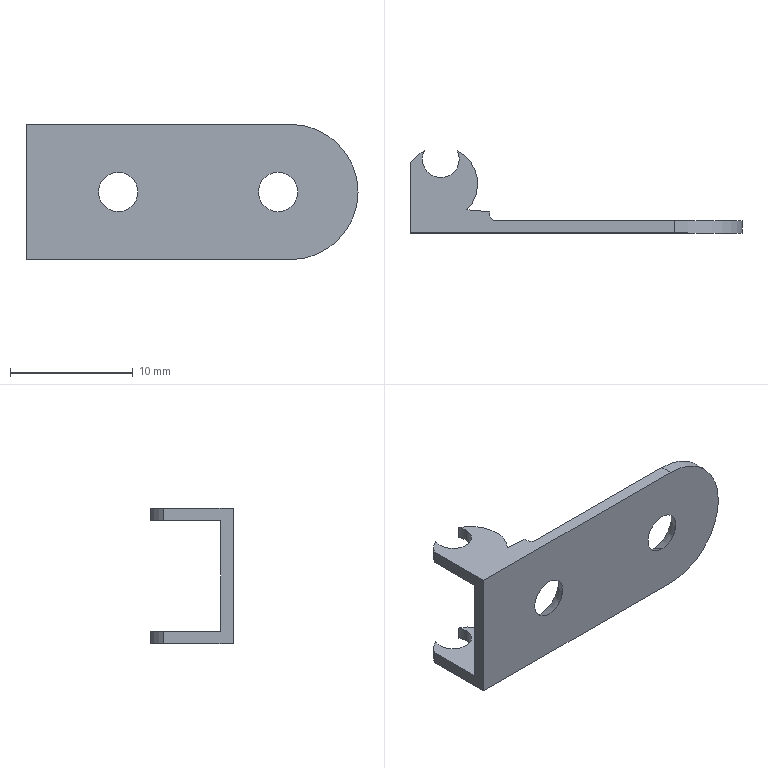Part | SolidWorks | features RefAxis 3, ICE 2, RevCut 2, 3DProfileFeature 1, Extrusion 1 | 1 solid | 28 faces | box 27 x 6.688 x 11 mm | volume 310.781 mm3 | cylinder 13 | plane 11 | cone 4 | commonest cylinder face diameters 3 x6 6 x4 1 x2 11 x1
STEP:
#1=CARTESIAN_POINT('',(20.5,0.,-1.6));
#2=VERTEX_POINT('',#1);
#3=CARTESIAN_POINT('',(20.5,0.,1.6));
#4=VERTEX_POINT('',#3);
#5=CARTESIAN_POINT('',(20.5,0.,0.));
#6=DIRECTION('',(0.,1.,0.));
#7=DIRECTION('',(0.,0.,1.));
#8=AXIS2_PLACEMENT_3D('',#5,#6,#7);
#9=CIRCLE('',#8,1.6);
#10=EDGE_CURVE('',#2,#4,#9,.T.);
#11=ORIENTED_EDGE('',*,*,#10,.F.);
#12=CARTESIAN_POINT('',(20.5,1.,-2.1));
#13=VERTEX_POINT('',#12);
#14=CARTESIAN_POINT('',(20.5,0.,-1.6));
#15=DIRECTION('',(0.,0.8944,-0.4472));
#16=VECTOR('',#15,1000.);
#17=LINE('',#14,#16);
#18=EDGE_CURVE('',#2,#13,#17,.T.);
#19=ORIENTED_EDGE('',*,*,#18,.T.);
#20=CARTESIAN_POINT('',(20.5,1.,2.1));
#21=VERTEX_POINT('',#20);
#22=CARTESIAN_POINT('',(20.5,1.,0.));
#23=DIRECTION('',(0.,1.,0.));
#24=DIRECTION('',(0.,0.,1.));
#25=AXIS2_PLACEMENT_3D('',#22,#23,#24);
#26=CIRCLE('',#25,2.1);
#27=EDGE_CURVE('',#13,#21,#26,.T.);
#28=ORIENTED_EDGE('',*,*,#27,.T.);
#29=CARTESIAN_POINT('',(20.5,0.,1.6));
#30=DIRECTION('',(0.,0.8944,0.4472));
#31=VECTOR('',#30,1000.);
#32=LINE('',#29,#31);
#33=EDGE_CURVE('',#4,#21,#32,.T.);
#34=ORIENTED_EDGE('',*,*,#33,.F.);
#35=EDGE_LOOP('',(#11,#19,#28,#34));
#36=FACE_OUTER_BOUND('',#35,.T.);
#37=CARTESIAN_POINT('',(20.5,0.,0.));
#38=DIRECTION('',(0.,1.,0.));
#39=DIRECTION('',(0.,0.,1.));
#40=AXIS2_PLACEMENT_3D('',#37,#38,#39);
#41=CONICAL_SURFACE('',#40,1.6,0.4636);
#42=ADVANCED_FACE('',(#36),#41,.F.);
#43=CARTESIAN_POINT('',(7.5,0.,-1.6));
#44=VERTEX_POINT('',#43);
#45=CARTESIAN_POINT('',(7.5,0.,1.6));
#46=VERTEX_POINT('',#45);
#47=CARTESIAN_POINT('',(7.5,0.,0.));
#48=DIRECTION('',(0.,1.,0.));
#49=DIRECTION('',(0.,0.,1.));
#50=AXIS2_PLACEMENT_3D('',#47,#48,#49);
#51=CIRCLE('',#50,1.6);
#52=EDGE_CURVE('',#44,#46,#51,.T.);
#53=ORIENTED_EDGE('',*,*,#52,.F.);
#54=CARTESIAN_POINT('',(7.5,1.,-2.1));
#55=VERTEX_POINT('',#54);
#56=CARTESIAN_POINT('',(7.5,0.,-1.6));
#57=DIRECTION('',(0.,0.8944,-0.4472));
#58=VECTOR('',#57,1000.);
#59=LINE('',#56,#58);
#60=EDGE_CURVE('',#44,#55,#59,.T.);
#61=ORIENTED_EDGE('',*,*,#60,.T.);
#62=CARTESIAN_POINT('',(7.5,1.,2.1));
#63=VERTEX_POINT('',#62);
#64=CARTESIAN_POINT('',(7.5,1.,0.));
#65=DIRECTION('',(0.,1.,0.));
#66=DIRECTION('',(0.,0.,1.));
#67=AXIS2_PLACEMENT_3D('',#64,#65,#66);
#68=CIRCLE('',#67,2.1);
#69=EDGE_CURVE('',#55,#63,#68,.T.);
#70=ORIENTED_EDGE('',*,*,#69,.T.);
#71=CARTESIAN_POINT('',(7.5,0.,1.6));
#72=DIRECTION('',(0.,0.8944,0.4472));
#73=VECTOR('',#72,1000.);
#74=LINE('',#71,#73);
#75=EDGE_CURVE('',#46,#63,#74,.T.);
#76=ORIENTED_EDGE('',*,*,#75,.F.);
#77=EDGE_LOOP('',(#53,#61,#70,#76));
#78=FACE_OUTER_BOUND('',#77,.T.);
#79=CARTESIAN_POINT('',(7.5,0.,0.));
#80=DIRECTION('',(0.,1.,0.));
#81=DIRECTION('',(0.,0.,1.));
#82=AXIS2_PLACEMENT_3D('',#79,#80,#81);
#83=CONICAL_SURFACE('',#82,1.6,0.4636);
#84=ADVANCED_FACE('',(#78),#83,.F.);
#85=CARTESIAN_POINT('',(4.,6.,-4.5));
#86=VERTEX_POINT('',#85);
#87=CARTESIAN_POINT('',(1.,6.,-4.5));
#88=VERTEX_POINT('',#87);
#89=CARTESIAN_POINT('',(2.5,6.,-4.5));
#90=DIRECTION('',(0.,0.,-1.));
#91=DIRECTION('',(1.,0.,0.));
#92=AXIS2_PLACEMENT_3D('',#89,#90,#91);
#93=CIRCLE('',#92,1.5);
#94=EDGE_CURVE('',#86,#88,#93,.T.);
#95=ORIENTED_EDGE('',*,*,#94,.F.);
#96=CARTESIAN_POINT('',(4.,6.,-5.5));
#97=VERTEX_POINT('',#96);
#98=CARTESIAN_POINT('',(4.,6.,5.5));
#99=DIRECTION('',(0.,0.,-1.));
#100=VECTOR('',#99,1000.);
#101=LINE('',#98,#100);
#102=EDGE_CURVE('',#86,#97,#101,.T.);
#103=ORIENTED_EDGE('',*,*,#102,.T.);
#104=CARTESIAN_POINT('',(1.,6.,-5.5));
#105=VERTEX_POINT('',#104);
#106=CARTESIAN_POINT('',(2.5,6.,-5.5));
#107=DIRECTION('',(0.,0.,-1.));
#108=DIRECTION('',(-1.,0.,0.));
#109=AXIS2_PLACEMENT_3D('',#106,#107,#108);
#110=CIRCLE('',#109,1.5);
#111=EDGE_CURVE('',#97,#105,#110,.T.);
#112=ORIENTED_EDGE('',*,*,#111,.T.);
#113=CARTESIAN_POINT('',(1.,6.,5.5));
#114=DIRECTION('',(0.,0.,-1.));
#115=VECTOR('',#114,1000.);
#116=LINE('',#113,#115);
#117=EDGE_CURVE('',#88,#105,#116,.T.);
#118=ORIENTED_EDGE('',*,*,#117,.F.);
#119=EDGE_LOOP('',(#95,#103,#112,#118));
#120=FACE_OUTER_BOUND('',#119,.T.);
#121=CARTESIAN_POINT('',(2.5,6.,5.5));
#122=DIRECTION('',(0.,0.,-1.));
#123=DIRECTION('',(-1.,0.,0.));
#124=AXIS2_PLACEMENT_3D('',#121,#122,#123);
#125=CYLINDRICAL_SURFACE('',#124,1.5);
#126=ADVANCED_FACE('',(#120),#125,.F.);
#127=CARTESIAN_POINT('',(1.167,6.688,-4.5));
#128=VERTEX_POINT('',#127);
#129=CARTESIAN_POINT('',(2.5,6.,-4.5));
#130=DIRECTION('',(0.,0.,-1.));
#131=DIRECTION('',(1.,0.,0.));
#132=AXIS2_PLACEMENT_3D('',#129,#130,#131);
#133=CIRCLE('',#132,1.5);
#134=EDGE_CURVE('',#88,#128,#133,.T.);
#135=ORIENTED_EDGE('',*,*,#134,.F.);
#136=ORIENTED_EDGE('',*,*,#117,.T.);
#137=CARTESIAN_POINT('',(1.167,6.688,-5.5));
#138=VERTEX_POINT('',#137);
#139=CARTESIAN_POINT('',(2.5,6.,-5.5));
#140=DIRECTION('',(0.,0.,-1.));
#141=DIRECTION('',(-1.,0.,0.));
#142=AXIS2_PLACEMENT_3D('',#139,#140,#141);
#143=CIRCLE('',#142,1.5);
#144=EDGE_CURVE('',#105,#138,#143,.T.);
#145=ORIENTED_EDGE('',*,*,#144,.T.);
#146=CARTESIAN_POINT('',(1.167,6.688,5.5));
#147=DIRECTION('',(0.,0.,-1.));
#148=VECTOR('',#147,1000.);
#149=LINE('',#146,#148);
#150=EDGE_CURVE('',#128,#138,#149,.T.);
#151=ORIENTED_EDGE('',*,*,#150,.F.);
#152=EDGE_LOOP('',(#135,#136,#145,#151));
#153=FACE_OUTER_BOUND('',#152,.T.);
#154=CARTESIAN_POINT('',(2.5,6.,5.5));
#155=DIRECTION('',(0.,0.,-1.));
#156=DIRECTION('',(-1.,0.,0.));
#157=AXIS2_PLACEMENT_3D('',#154,#155,#156);
#158=CYLINDRICAL_SURFACE('',#157,1.5);
#159=ADVANCED_FACE('',(#153),#158,.F.);
#160=CARTESIAN_POINT('',(4.,6.,5.5));
#161=VERTEX_POINT('',#160);
#162=CARTESIAN_POINT('',(1.,6.,5.5));
#163=VERTEX_POINT('',#162);
#164=CARTESIAN_POINT('',(2.5,6.,5.5));
#165=DIRECTION('',(0.,0.,-1.));
#166=DIRECTION('',(-1.,0.,0.));
#167=AXIS2_PLACEMENT_3D('',#164,#165,#166);
#168=CIRCLE('',#167,1.5);
#169=EDGE_CURVE('',#161,#163,#168,.T.);
#170=ORIENTED_EDGE('',*,*,#169,.F.);
#171=CARTESIAN_POINT('',(4.,6.,4.5));
#172=VERTEX_POINT('',#171);
#173=CARTESIAN_POINT('',(4.,6.,5.5));
#174=DIRECTION('',(0.,0.,-1.));
#175=VECTOR('',#174,1000.);
#176=LINE('',#173,#175);
#177=EDGE_CURVE('',#161,#172,#176,.T.);
#178=ORIENTED_EDGE('',*,*,#177,.T.);
#179=CARTESIAN_POINT('',(1.,6.,4.5));
#180=VERTEX_POINT('',#179);
#181=CARTESIAN_POINT('',(2.5,6.,4.5));
#182=DIRECTION('',(0.,0.,1.));
#183=DIRECTION('',(-1.,0.,0.));
#184=AXIS2_PLACEMENT_3D('',#181,#182,#183);
#185=CIRCLE('',#184,1.5);
#186=EDGE_CURVE('',#180,#172,#185,.T.);
#187=ORIENTED_EDGE('',*,*,#186,.F.);
#188=CARTESIAN_POINT('',(1.,6.,5.5));
#189=DIRECTION('',(0.,0.,-1.));
#190=VECTOR('',#189,1000.);
#191=LINE('',#188,#190);
#192=EDGE_CURVE('',#163,#180,#191,.T.);
#193=ORIENTED_EDGE('',*,*,#192,.F.);
#194=EDGE_LOOP('',(#170,#178,#187,#193));
#195=FACE_OUTER_BOUND('',#194,.T.);
#196=CARTESIAN_POINT('',(2.5,6.,5.5));
#197=DIRECTION('',(0.,0.,-1.));
#198=DIRECTION('',(-1.,0.,0.));
#199=AXIS2_PLACEMENT_3D('',#196,#197,#198);
#200=CYLINDRICAL_SURFACE('',#199,1.5);
#201=ADVANCED_FACE('',(#195),#200,.F.);
#202=CARTESIAN_POINT('',(1.167,6.688,5.5));
#203=VERTEX_POINT('',#202);
#204=CARTESIAN_POINT('',(2.5,6.,5.5));
#205=DIRECTION('',(0.,0.,-1.));
#206=DIRECTION('',(-1.,0.,0.));
#207=AXIS2_PLACEMENT_3D('',#204,#205,#206);
#208=CIRCLE('',#207,1.5);
#209=EDGE_CURVE('',#163,#203,#208,.T.);
#210=ORIENTED_EDGE('',*,*,#209,.F.);
#211=ORIENTED_EDGE('',*,*,#192,.T.);
#212=CARTESIAN_POINT('',(1.167,6.687,4.5));
#213=VERTEX_POINT('',#212);
#214=CARTESIAN_POINT('',(2.5,6.,4.5));
#215=DIRECTION('',(0.,0.,1.));
#216=DIRECTION('',(-1.,0.,0.));
#217=AXIS2_PLACEMENT_3D('',#214,#215,#216);
#218=CIRCLE('',#217,1.5);
#219=EDGE_CURVE('',#213,#180,#218,.T.);
#220=ORIENTED_EDGE('',*,*,#219,.F.);
#221=CARTESIAN_POINT('',(1.167,6.688,5.5));
#222=DIRECTION('',(0.,0.,-1.));
#223=VECTOR('',#222,1000.);
#224=LINE('',#221,#223);
#225=EDGE_CURVE('',#203,#213,#224,.T.);
#226=ORIENTED_EDGE('',*,*,#225,.F.);
#227=EDGE_LOOP('',(#210,#211,#220,#226));
#228=FACE_OUTER_BOUND('',#227,.T.);
#229=CARTESIAN_POINT('',(2.5,6.,5.5));
#230=DIRECTION('',(0.,0.,-1.));
#231=DIRECTION('',(-1.,0.,0.));
#232=AXIS2_PLACEMENT_3D('',#229,#230,#231);
#233=CYLINDRICAL_SURFACE('',#232,1.5);
#234=ADVANCED_FACE('',(#228),#233,.F.);
#235=CARTESIAN_POINT('',(7.5,0.,0.));
#236=DIRECTION('',(0.,1.,0.));
#237=DIRECTION('',(0.,0.,1.));
#238=AXIS2_PLACEMENT_3D('',#235,#236,#237);
#239=CIRCLE('',#238,1.6);
#240=EDGE_CURVE('',#46,#44,#239,.T.);
#241=ORIENTED_EDGE('',*,*,#240,.T.);
#242=ORIENTED_EDGE('',*,*,#52,.T.);
#243=EDGE_LOOP('',(#241,#242));
#244=FACE_BOUND('',#243,.T.);
#245=CARTESIAN_POINT('',(0.,0.,-5.5));
#246=VERTEX_POINT('',#245);
#247=CARTESIAN_POINT('',(21.5,0.,-5.5));
#248=VERTEX_POINT('',#247);
#249=CARTESIAN_POINT('',(0.,0.,-5.5));
#250=DIRECTION('',(1.,0.,0.));
#251=VECTOR('',#250,1000.);
#252=LINE('',#249,#251);
#253=EDGE_CURVE('',#246,#248,#252,.T.);
#254=ORIENTED_EDGE('',*,*,#253,.T.);
#255=CARTESIAN_POINT('',(21.5,0.,5.5));
#256=VERTEX_POINT('',#255);
#257=CARTESIAN_POINT('',(21.5,0.,0.));
#258=DIRECTION('',(0.,1.,0.));
#259=DIRECTION('',(0.,0.,1.));
#260=AXIS2_PLACEMENT_3D('',#257,#258,#259);
#261=CIRCLE('',#260,5.5);
#262=EDGE_CURVE('',#256,#248,#261,.T.);
#263=ORIENTED_EDGE('',*,*,#262,.F.);
#264=CARTESIAN_POINT('',(0.,0.,5.5));
#265=VERTEX_POINT('',#264);
#266=CARTESIAN_POINT('',(0.,0.,5.5));
#267=DIRECTION('',(1.,0.,0.));
#268=VECTOR('',#267,1000.);
#269=LINE('',#266,#268);
#270=EDGE_CURVE('',#265,#256,#269,.T.);
#271=ORIENTED_EDGE('',*,*,#270,.F.);
#272=CARTESIAN_POINT('',(0.,0.,5.5));
#273=DIRECTION('',(0.,0.,-1.));
#274=VECTOR('',#273,1000.);
#275=LINE('',#272,#274);
#276=EDGE_CURVE('',#265,#246,#275,.T.);
#277=ORIENTED_EDGE('',*,*,#276,.T.);
#278=EDGE_LOOP('',(#254,#263,#271,#277));
#279=FACE_OUTER_BOUND('',#278,.T.);
#280=CARTESIAN_POINT('',(20.5,0.,0.));
#281=DIRECTION('',(0.,1.,0.));
#282=DIRECTION('',(0.,0.,1.));
#283=AXIS2_PLACEMENT_3D('',#280,#281,#282);
#284=CIRCLE('',#283,1.6);
#285=EDGE_CURVE('',#4,#2,#284,.T.);
#286=ORIENTED_EDGE('',*,*,#285,.T.);
#287=ORIENTED_EDGE('',*,*,#10,.T.);
#288=EDGE_LOOP('',(#286,#287));
#289=FACE_BOUND('',#288,.T.);
#290=CARTESIAN_POINT('',(0.,0.,5.5));
#291=DIRECTION('',(0.,1.,0.));
#292=DIRECTION('',(0.,0.,1.));
#293=AXIS2_PLACEMENT_3D('',#290,#291,#292);
#294=PLANE('',#293);
#295=ADVANCED_FACE('',(#244,#279,#289),#294,.F.);
#296=CARTESIAN_POINT('',(7.5,1.,0.));
#297=DIRECTION('',(0.,1.,0.));
#298=DIRECTION('',(0.,0.,1.));
#299=AXIS2_PLACEMENT_3D('',#296,#297,#298);
#300=CIRCLE('',#299,2.1);
#301=EDGE_CURVE('',#63,#55,#300,.T.);
#302=ORIENTED_EDGE('',*,*,#301,.F.);
#303=ORIENTED_EDGE('',*,*,#69,.F.);
#304=EDGE_LOOP('',(#302,#303));
#305=FACE_BOUND('',#304,.T.);
#306=CARTESIAN_POINT('',(6.99,1.,-4.5));
#307=VERTEX_POINT('',#306);
#308=CARTESIAN_POINT('',(6.99,1.,-5.5));
#309=VERTEX_POINT('',#308);
#310=CARTESIAN_POINT('',(6.99,1.,5.5));
#311=DIRECTION('',(0.,0.,-1.));
#312=VECTOR('',#311,1000.);
#313=LINE('',#310,#312);
#314=EDGE_CURVE('',#307,#309,#313,.T.);
#315=ORIENTED_EDGE('',*,*,#314,.F.);
#316=CARTESIAN_POINT('',(0.,1.,-4.5));
#317=VERTEX_POINT('',#316);
#318=CARTESIAN_POINT('',(11.,1.,-4.5));
#319=DIRECTION('',(-1.,0.,0.));
#320=VECTOR('',#319,1000.);
#321=LINE('',#318,#320);
#322=EDGE_CURVE('',#307,#317,#321,.T.);
#323=ORIENTED_EDGE('',*,*,#322,.T.);
#324=CARTESIAN_POINT('',(0.,1.,4.5));
#325=VERTEX_POINT('',#324);
#326=CARTESIAN_POINT('',(0.,1.,4.5));
#327=DIRECTION('',(0.,0.,-1.));
#328=VECTOR('',#327,1000.);
#329=LINE('',#326,#328);
#330=EDGE_CURVE('',#325,#317,#329,.T.);
#331=ORIENTED_EDGE('',*,*,#330,.F.);
#332=CARTESIAN_POINT('',(6.99,1.,4.5));
#333=VERTEX_POINT('',#332);
#334=CARTESIAN_POINT('',(11.,1.,4.5));
#335=DIRECTION('',(-1.,0.,0.));
#336=VECTOR('',#335,1000.);
#337=LINE('',#334,#336);
#338=EDGE_CURVE('',#333,#325,#337,.T.);
#339=ORIENTED_EDGE('',*,*,#338,.F.);
#340=CARTESIAN_POINT('',(6.99,1.,5.5));
#341=VERTEX_POINT('',#340);
#342=CARTESIAN_POINT('',(6.99,1.,5.5));
#343=DIRECTION('',(0.,0.,-1.));
#344=VECTOR('',#343,1000.);
#345=LINE('',#342,#344);
#346=EDGE_CURVE('',#341,#333,#345,.T.);
#347=ORIENTED_EDGE('',*,*,#346,.F.);
#348=CARTESIAN_POINT('',(21.5,1.,5.5));
#349=VERTEX_POINT('',#348);
#350=CARTESIAN_POINT('',(27.,1.,5.5));
#351=DIRECTION('',(-1.,0.,0.));
#352=VECTOR('',#351,1000.);
#353=LINE('',#350,#352);
#354=EDGE_CURVE('',#349,#341,#353,.T.);
#355=ORIENTED_EDGE('',*,*,#354,.F.);
#356=CARTESIAN_POINT('',(21.5,1.,-5.5));
#357=VERTEX_POINT('',#356);
#358=CARTESIAN_POINT('',(21.5,1.,0.));
#359=DIRECTION('',(0.,1.,0.));
#360=DIRECTION('',(0.,0.,-1.));
#361=AXIS2_PLACEMENT_3D('',#358,#359,#360);
#362=CIRCLE('',#361,5.5);
#363=EDGE_CURVE('',#349,#357,#362,.T.);
#364=ORIENTED_EDGE('',*,*,#363,.T.);
#365=CARTESIAN_POINT('',(27.,1.,-5.5));
#366=DIRECTION('',(-1.,0.,0.));
#367=VECTOR('',#366,1000.);
#368=LINE('',#365,#367);
#369=EDGE_CURVE('',#357,#309,#368,.T.);
#370=ORIENTED_EDGE('',*,*,#369,.T.);
#371=EDGE_LOOP('',(#315,#323,#331,#339,#347,#355,#364,#370));
#372=FACE_OUTER_BOUND('',#371,.T.);
#373=CARTESIAN_POINT('',(20.5,1.,0.));
#374=DIRECTION('',(0.,1.,0.));
#375=DIRECTION('',(0.,0.,1.));
#376=AXIS2_PLACEMENT_3D('',#373,#374,#375);
#377=CIRCLE('',#376,2.1);
#378=EDGE_CURVE('',#21,#13,#377,.T.);
#379=ORIENTED_EDGE('',*,*,#378,.F.);
#380=ORIENTED_EDGE('',*,*,#27,.F.);
#381=EDGE_LOOP('',(#379,#380));
#382=FACE_BOUND('',#381,.T.);
#383=CARTESIAN_POINT('',(27.,1.,5.5));
#384=DIRECTION('',(0.,-1.,0.));
#385=DIRECTION('',(0.,0.,-1.));
#386=AXIS2_PLACEMENT_3D('',#383,#384,#385);
#387=PLANE('',#386);
#388=ADVANCED_FACE('',(#305,#372,#382),#387,.F.);
#389=CARTESIAN_POINT('',(0.,5.658,4.5));
#390=VERTEX_POINT('',#389);
#391=CARTESIAN_POINT('',(0.,11.,4.5));
#392=DIRECTION('',(0.,-1.,0.));
#393=VECTOR('',#392,1000.);
#394=LINE('',#391,#393);
#395=EDGE_CURVE('',#390,#325,#394,.T.);
#396=ORIENTED_EDGE('',*,*,#395,.T.);
#397=ORIENTED_EDGE('',*,*,#330,.T.);
#398=CARTESIAN_POINT('',(0.,5.658,-4.5));
#399=VERTEX_POINT('',#398);
#400=CARTESIAN_POINT('',(0.,1.,-4.5));
#401=DIRECTION('',(0.,1.,0.));
#402=VECTOR('',#401,1000.);
#403=LINE('',#400,#402);
#404=EDGE_CURVE('',#317,#399,#403,.T.);
#405=ORIENTED_EDGE('',*,*,#404,.T.);
#406=CARTESIAN_POINT('',(0.,5.658,-5.5));
#407=VERTEX_POINT('',#406);
#408=CARTESIAN_POINT('',(0.,5.658,5.5));
#409=DIRECTION('',(0.,0.,-1.));
#410=VECTOR('',#409,1000.);
#411=LINE('',#408,#410);
#412=EDGE_CURVE('',#399,#407,#411,.T.);
#413=ORIENTED_EDGE('',*,*,#412,.T.);
#414=CARTESIAN_POINT('',(0.,5.658,-5.5));
#415=DIRECTION('',(0.,-1.,0.));
#416=VECTOR('',#415,1000.);
#417=LINE('',#414,#416);
#418=EDGE_CURVE('',#407,#246,#417,.T.);
#419=ORIENTED_EDGE('',*,*,#418,.T.);
#420=ORIENTED_EDGE('',*,*,#276,.F.);
#421=CARTESIAN_POINT('',(0.,5.658,5.5));
#422=VERTEX_POINT('',#421);
#423=CARTESIAN_POINT('',(0.,5.658,5.5));
#424=DIRECTION('',(0.,-1.,0.));
#425=VECTOR('',#424,1000.);
#426=LINE('',#423,#425);
#427=EDGE_CURVE('',#422,#265,#426,.T.);
#428=ORIENTED_EDGE('',*,*,#427,.F.);
#429=CARTESIAN_POINT('',(0.,5.658,5.5));
#430=DIRECTION('',(0.,0.,-1.));
#431=VECTOR('',#430,1000.);
#432=LINE('',#429,#431);
#433=EDGE_CURVE('',#422,#390,#432,.T.);
#434=ORIENTED_EDGE('',*,*,#433,.T.);
#435=EDGE_LOOP('',(#396,#397,#405,#413,#419,#420,#428,#434));
#436=FACE_OUTER_BOUND('',#435,.T.);
#437=CARTESIAN_POINT('',(0.,5.658,5.5));
#438=DIRECTION('',(1.,0.,0.));
#439=DIRECTION('',(0.,0.,-1.));
#440=AXIS2_PLACEMENT_3D('',#437,#438,#439);
#441=PLANE('',#440);
#442=ADVANCED_FACE('',(#436),#441,.F.);
#443=CARTESIAN_POINT('',(6.49,1.5,4.5));
#444=VERTEX_POINT('',#443);
#445=CARTESIAN_POINT('',(6.99,1.5,4.5));
#446=DIRECTION('',(0.,0.,1.));
#447=DIRECTION('',(-1.,0.,0.));
#448=AXIS2_PLACEMENT_3D('',#445,#446,#447);
#449=CIRCLE('',#448,0.5);
#450=EDGE_CURVE('',#444,#333,#449,.T.);
#451=ORIENTED_EDGE('',*,*,#450,.F.);
#452=CARTESIAN_POINT('',(6.49,1.5,5.5));
#453=VERTEX_POINT('',#452);
#454=CARTESIAN_POINT('',(6.49,1.5,5.5));
#455=DIRECTION('',(0.,0.,-1.));
#456=VECTOR('',#455,1000.);
#457=LINE('',#454,#456);
#458=EDGE_CURVE('',#453,#444,#457,.T.);
#459=ORIENTED_EDGE('',*,*,#458,.F.);
#460=CARTESIAN_POINT('',(6.99,1.5,5.5));
#461=DIRECTION('',(0.,0.,-1.));
#462=DIRECTION('',(-1.,0.,0.));
#463=AXIS2_PLACEMENT_3D('',#460,#461,#462);
#464=CIRCLE('',#463,0.5);
#465=EDGE_CURVE('',#341,#453,#464,.T.);
#466=ORIENTED_EDGE('',*,*,#465,.F.);
#467=ORIENTED_EDGE('',*,*,#346,.T.);
#468=EDGE_LOOP('',(#451,#459,#466,#467));
#469=FACE_OUTER_BOUND('',#468,.T.);
#470=CARTESIAN_POINT('',(6.99,1.5,5.5));
#471=DIRECTION('',(0.,0.,-1.));
#472=DIRECTION('',(-1.,0.,0.));
#473=AXIS2_PLACEMENT_3D('',#470,#471,#472);
#474=CYLINDRICAL_SURFACE('',#473,0.5);
#475=ADVANCED_FACE('',(#469),#474,.F.);
#476=CARTESIAN_POINT('',(6.49,1.5,-4.5));
#477=VERTEX_POINT('',#476);
#478=CARTESIAN_POINT('',(6.99,1.5,-4.5));
#479=DIRECTION('',(0.,0.,-1.));
#480=DIRECTION('',(1.,0.,0.));
#481=AXIS2_PLACEMENT_3D('',#478,#479,#480);
#482=CIRCLE('',#481,0.5);
#483=EDGE_CURVE('',#307,#477,#482,.T.);
#484=ORIENTED_EDGE('',*,*,#483,.F.);
#485=ORIENTED_EDGE('',*,*,#314,.T.);
#486=CARTESIAN_POINT('',(6.49,1.5,-5.5));
#487=VERTEX_POINT('',#486);
#488=CARTESIAN_POINT('',(6.99,1.5,-5.5));
#489=DIRECTION('',(0.,0.,-1.));
#490=DIRECTION('',(-1.,0.,0.));
#491=AXIS2_PLACEMENT_3D('',#488,#489,#490);
#492=CIRCLE('',#491,0.5);
#493=EDGE_CURVE('',#309,#487,#492,.T.);
#494=ORIENTED_EDGE('',*,*,#493,.T.);
#495=CARTESIAN_POINT('',(6.49,1.5,5.5));
#496=DIRECTION('',(0.,0.,-1.));
#497=VECTOR('',#496,1000.);
#498=LINE('',#495,#497);
#499=EDGE_CURVE('',#477,#487,#498,.T.);
#500=ORIENTED_EDGE('',*,*,#499,.F.);
#501=EDGE_LOOP('',(#484,#485,#494,#500));
#502=FACE_OUTER_BOUND('',#501,.T.);
#503=CARTESIAN_POINT('',(6.99,1.5,5.5));
#504=DIRECTION('',(0.,0.,-1.));
#505=DIRECTION('',(-1.,0.,0.));
#506=AXIS2_PLACEMENT_3D('',#503,#504,#505);
#507=CYLINDRICAL_SURFACE('',#506,0.5);
#508=ADVANCED_FACE('',(#502),#507,.F.);
#509=CARTESIAN_POINT('',(6.49,1.725,4.5));
#510=VERTEX_POINT('',#509);
#511=CARTESIAN_POINT('',(6.49,1.5,4.5));
#512=DIRECTION('',(0.,-1.,0.));
#513=VECTOR('',#512,1000.);
#514=LINE('',#511,#513);
#515=EDGE_CURVE('',#510,#444,#514,.T.);
#516=ORIENTED_EDGE('',*,*,#515,.F.);
#517=CARTESIAN_POINT('',(6.49,1.725,5.5));
#518=VERTEX_POINT('',#517);
#519=CARTESIAN_POINT('',(6.49,1.725,5.5));
#520=DIRECTION('',(0.,0.,-1.));
#521=VECTOR('',#520,1000.);
#522=LINE('',#519,#521);
#523=EDGE_CURVE('',#518,#510,#522,.T.);
#524=ORIENTED_EDGE('',*,*,#523,.F.);
#525=CARTESIAN_POINT('',(6.49,1.5,5.5));
#526=DIRECTION('',(0.,1.,0.));
#527=VECTOR('',#526,1000.);
#528=LINE('',#525,#527);
#529=EDGE_CURVE('',#453,#518,#528,.T.);
#530=ORIENTED_EDGE('',*,*,#529,.F.);
#531=ORIENTED_EDGE('',*,*,#458,.T.);
#532=EDGE_LOOP('',(#516,#524,#530,#531));
#533=FACE_OUTER_BOUND('',#532,.T.);
#534=CARTESIAN_POINT('',(6.49,1.5,5.5));
#535=DIRECTION('',(-1.,0.,0.));
#536=DIRECTION('',(0.,0.,1.));
#537=AXIS2_PLACEMENT_3D('',#534,#535,#536);
#538=PLANE('',#537);
#539=ADVANCED_FACE('',(#533),#538,.F.);
#540=CARTESIAN_POINT('',(6.49,1.725,-4.5));
#541=VERTEX_POINT('',#540);
#542=CARTESIAN_POINT('',(6.49,1.5,-4.5));
#543=DIRECTION('',(0.,1.,0.));
#544=VECTOR('',#543,1000.);
#545=LINE('',#542,#544);
#546=EDGE_CURVE('',#477,#541,#545,.T.);
#547=ORIENTED_EDGE('',*,*,#546,.F.);
#548=ORIENTED_EDGE('',*,*,#499,.T.);
#549=CARTESIAN_POINT('',(6.49,1.725,-5.5));
#550=VERTEX_POINT('',#549);
#551=CARTESIAN_POINT('',(6.49,1.5,-5.5));
#552=DIRECTION('',(0.,1.,0.));
#553=VECTOR('',#552,1000.);
#554=LINE('',#551,#553);
#555=EDGE_CURVE('',#487,#550,#554,.T.);
#556=ORIENTED_EDGE('',*,*,#555,.T.);
#557=CARTESIAN_POINT('',(6.49,1.725,5.5));
#558=DIRECTION('',(0.,0.,-1.));
#559=VECTOR('',#558,1000.);
#560=LINE('',#557,#559);
#561=EDGE_CURVE('',#541,#550,#560,.T.);
#562=ORIENTED_EDGE('',*,*,#561,.F.);
#563=EDGE_LOOP('',(#547,#548,#556,#562));
#564=FACE_OUTER_BOUND('',#563,.T.);
#565=CARTESIAN_POINT('',(6.49,1.5,5.5));
#566=DIRECTION('',(-1.,0.,0.));
#567=DIRECTION('',(0.,0.,1.));
#568=AXIS2_PLACEMENT_3D('',#565,#566,#567);
#569=PLANE('',#568);
#570=ADVANCED_FACE('',(#564),#569,.F.);
#571=CARTESIAN_POINT('',(4.63,1.887,4.5));
#572=VERTEX_POINT('',#571);
#573=CARTESIAN_POINT('',(6.49,1.725,4.5));
#574=DIRECTION('',(0.9962,-0.08716,0.));
#575=VECTOR('',#574,1000.);
#576=LINE('',#573,#575);
#577=EDGE_CURVE('',#572,#510,#576,.T.);
#578=ORIENTED_EDGE('',*,*,#577,.F.);
#579=CARTESIAN_POINT('',(4.63,1.887,5.5));
#580=VERTEX_POINT('',#579);
#581=CARTESIAN_POINT('',(4.63,1.887,5.5));
#582=DIRECTION('',(0.,0.,-1.));
#583=VECTOR('',#582,1000.);
#584=LINE('',#581,#583);
#585=EDGE_CURVE('',#580,#572,#584,.T.);
#586=ORIENTED_EDGE('',*,*,#585,.F.);
#587=CARTESIAN_POINT('',(6.49,1.725,5.5));
#588=DIRECTION('',(-0.9962,0.08716,0.));
#589=VECTOR('',#588,1000.);
#590=LINE('',#587,#589);
#591=EDGE_CURVE('',#518,#580,#590,.T.);
#592=ORIENTED_EDGE('',*,*,#591,.F.);
#593=ORIENTED_EDGE('',*,*,#523,.T.);
#594=EDGE_LOOP('',(#578,#586,#592,#593));
#595=FACE_OUTER_BOUND('',#594,.T.);
#596=CARTESIAN_POINT('',(6.49,1.725,5.5));
#597=DIRECTION('',(-0.08716,-0.9962,0.));
#598=DIRECTION('',(0.9962,-0.08716,0.));
#599=AXIS2_PLACEMENT_3D('',#596,#597,#598);
#600=PLANE('',#599);
#601=ADVANCED_FACE('',(#595),#600,.F.);
#602=CARTESIAN_POINT('',(4.63,1.887,-4.5));
#603=VERTEX_POINT('',#602);
#604=CARTESIAN_POINT('',(6.49,1.725,-4.5));
#605=DIRECTION('',(-0.9962,0.08716,0.));
#606=VECTOR('',#605,1000.);
#607=LINE('',#604,#606);
#608=EDGE_CURVE('',#541,#603,#607,.T.);
#609=ORIENTED_EDGE('',*,*,#608,.F.);
#610=ORIENTED_EDGE('',*,*,#561,.T.);
#611=CARTESIAN_POINT('',(4.63,1.887,-5.5));
#612=VERTEX_POINT('',#611);
#613=CARTESIAN_POINT('',(6.49,1.725,-5.5));
#614=DIRECTION('',(-0.9962,0.08716,0.));
#615=VECTOR('',#614,1000.);
#616=LINE('',#613,#615);
#617=EDGE_CURVE('',#550,#612,#616,.T.);
#618=ORIENTED_EDGE('',*,*,#617,.T.);
#619=CARTESIAN_POINT('',(4.63,1.887,5.5));
#620=DIRECTION('',(0.,0.,-1.));
#621=VECTOR('',#620,1000.);
#622=LINE('',#619,#621);
#623=EDGE_CURVE('',#603,#612,#622,.T.);
#624=ORIENTED_EDGE('',*,*,#623,.F.);
#625=EDGE_LOOP('',(#609,#610,#618,#624));
#626=FACE_OUTER_BOUND('',#625,.T.);
#627=CARTESIAN_POINT('',(6.49,1.725,5.5));
#628=DIRECTION('',(-0.08716,-0.9962,0.));
#629=DIRECTION('',(0.9962,-0.08716,0.));
#630=AXIS2_PLACEMENT_3D('',#627,#628,#629);
#631=PLANE('',#630);
#632=ADVANCED_FACE('',(#626),#631,.F.);
#633=CARTESIAN_POINT('',(3.833,6.687,4.5));
#634=VERTEX_POINT('',#633);
#635=CARTESIAN_POINT('',(2.5,4.,4.5));
#636=DIRECTION('',(0.,0.,-1.));
#637=DIRECTION('',(-1.,0.,0.));
#638=AXIS2_PLACEMENT_3D('',#635,#636,#637);
#639=CIRCLE('',#638,3.);
#640=EDGE_CURVE('',#634,#572,#639,.T.);
#641=ORIENTED_EDGE('',*,*,#640,.F.);
#642=CARTESIAN_POINT('',(3.833,6.687,5.5));
#643=VERTEX_POINT('',#642);
#644=CARTESIAN_POINT('',(3.833,6.687,5.5));
#645=DIRECTION('',(0.,0.,-1.));
#646=VECTOR('',#645,1000.);
#647=LINE('',#644,#646);
#648=EDGE_CURVE('',#643,#634,#647,.T.);
#649=ORIENTED_EDGE('',*,*,#648,.F.);
#650=CARTESIAN_POINT('',(2.5,4.,5.5));
#651=DIRECTION('',(0.,0.,1.));
#652=DIRECTION('',(1.,0.,0.));
#653=AXIS2_PLACEMENT_3D('',#650,#651,#652);
#654=CIRCLE('',#653,3.);
#655=EDGE_CURVE('',#580,#643,#654,.T.);
#656=ORIENTED_EDGE('',*,*,#655,.F.);
#657=ORIENTED_EDGE('',*,*,#585,.T.);
#658=EDGE_LOOP('',(#641,#649,#656,#657));
#659=FACE_OUTER_BOUND('',#658,.T.);
#660=CARTESIAN_POINT('',(2.5,4.,5.5));
#661=DIRECTION('',(0.,0.,-1.));
#662=DIRECTION('',(-1.,0.,0.));
#663=AXIS2_PLACEMENT_3D('',#660,#661,#662);
#664=CYLINDRICAL_SURFACE('',#663,3.);
#665=ADVANCED_FACE('',(#659),#664,.T.);
#666=CARTESIAN_POINT('',(3.833,6.687,-4.5));
#667=VERTEX_POINT('',#666);
#668=CARTESIAN_POINT('',(2.5,4.,-4.5));
#669=DIRECTION('',(0.,0.,1.));
#670=DIRECTION('',(1.,0.,0.));
#671=AXIS2_PLACEMENT_3D('',#668,#669,#670);
#672=CIRCLE('',#671,3.);
#673=EDGE_CURVE('',#603,#667,#672,.T.);
#674=ORIENTED_EDGE('',*,*,#673,.F.);
#675=ORIENTED_EDGE('',*,*,#623,.T.);
#676=CARTESIAN_POINT('',(3.833,6.687,-5.5));
#677=VERTEX_POINT('',#676);
#678=CARTESIAN_POINT('',(2.5,4.,-5.5));
#679=DIRECTION('',(0.,0.,1.));
#680=DIRECTION('',(1.,0.,0.));
#681=AXIS2_PLACEMENT_3D('',#678,#679,#680);
#682=CIRCLE('',#681,3.);
#683=EDGE_CURVE('',#612,#677,#682,.T.);
#684=ORIENTED_EDGE('',*,*,#683,.T.);
#685=CARTESIAN_POINT('',(3.833,6.687,5.5));
#686=DIRECTION('',(0.,0.,-1.));
#687=VECTOR('',#686,1000.);
#688=LINE('',#685,#687);
#689=EDGE_CURVE('',#667,#677,#688,.T.);
#690=ORIENTED_EDGE('',*,*,#689,.F.);
#691=EDGE_LOOP('',(#674,#675,#684,#690));
#692=FACE_OUTER_BOUND('',#691,.T.);
#693=CARTESIAN_POINT('',(2.5,4.,5.5));
#694=DIRECTION('',(0.,0.,-1.));
#695=DIRECTION('',(-1.,0.,0.));
#696=AXIS2_PLACEMENT_3D('',#693,#694,#695);
#697=CYLINDRICAL_SURFACE('',#696,3.);
#698=ADVANCED_FACE('',(#692),#697,.T.);
#699=ORIENTED_EDGE('',*,*,#177,.F.);
#700=CARTESIAN_POINT('',(2.5,6.,5.5));
#701=DIRECTION('',(0.,0.,-1.));
#702=DIRECTION('',(-1.,0.,0.));
#703=AXIS2_PLACEMENT_3D('',#700,#701,#702);
#704=CIRCLE('',#703,1.5);
#705=EDGE_CURVE('',#643,#161,#704,.T.);
#706=ORIENTED_EDGE('',*,*,#705,.F.);
#707=ORIENTED_EDGE('',*,*,#648,.T.);
#708=CARTESIAN_POINT('',(2.5,6.,4.5));
#709=DIRECTION('',(0.,0.,1.));
#710=DIRECTION('',(-1.,0.,0.));
#711=AXIS2_PLACEMENT_3D('',#708,#709,#710);
#712=CIRCLE('',#711,1.5);
#713=EDGE_CURVE('',#172,#634,#712,.T.);
#714=ORIENTED_EDGE('',*,*,#713,.F.);
#715=EDGE_LOOP('',(#699,#706,#707,#714));
#716=FACE_OUTER_BOUND('',#715,.T.);
#717=CARTESIAN_POINT('',(2.5,6.,5.5));
#718=DIRECTION('',(0.,0.,-1.));
#719=DIRECTION('',(-1.,0.,0.));
#720=AXIS2_PLACEMENT_3D('',#717,#718,#719);
#721=CYLINDRICAL_SURFACE('',#720,1.5);
#722=ADVANCED_FACE('',(#716),#721,.F.);
#723=ORIENTED_EDGE('',*,*,#102,.F.);
#724=CARTESIAN_POINT('',(2.5,6.,-4.5));
#725=DIRECTION('',(0.,0.,-1.));
#726=DIRECTION('',(1.,0.,0.));
#727=AXIS2_PLACEMENT_3D('',#724,#725,#726);
#728=CIRCLE('',#727,1.5);
#729=EDGE_CURVE('',#667,#86,#728,.T.);
#730=ORIENTED_EDGE('',*,*,#729,.F.);
#731=ORIENTED_EDGE('',*,*,#689,.T.);
#732=CARTESIAN_POINT('',(2.5,6.,-5.5));
#733=DIRECTION('',(0.,0.,-1.));
#734=DIRECTION('',(-1.,0.,0.));
#735=AXIS2_PLACEMENT_3D('',#732,#733,#734);
#736=CIRCLE('',#735,1.5);
#737=EDGE_CURVE('',#677,#97,#736,.T.);
#738=ORIENTED_EDGE('',*,*,#737,.T.);
#739=EDGE_LOOP('',(#723,#730,#731,#738));
#740=FACE_OUTER_BOUND('',#739,.T.);
#741=CARTESIAN_POINT('',(2.5,6.,5.5));
#742=DIRECTION('',(0.,0.,-1.));
#743=DIRECTION('',(-1.,0.,0.));
#744=AXIS2_PLACEMENT_3D('',#741,#742,#743);
#745=CYLINDRICAL_SURFACE('',#744,1.5);
#746=ADVANCED_FACE('',(#740),#745,.F.);
#747=CARTESIAN_POINT('',(2.5,4.,4.5));
#748=DIRECTION('',(0.,0.,-1.));
#749=DIRECTION('',(-1.,0.,0.));
#750=AXIS2_PLACEMENT_3D('',#747,#748,#749);
#751=CIRCLE('',#750,3.);
#752=EDGE_CURVE('',#390,#213,#751,.T.);
#753=ORIENTED_EDGE('',*,*,#752,.F.);
#754=ORIENTED_EDGE('',*,*,#433,.F.);
#755=CARTESIAN_POINT('',(2.5,4.,5.5));
#756=DIRECTION('',(0.,0.,1.));
#757=DIRECTION('',(1.,0.,0.));
#758=AXIS2_PLACEMENT_3D('',#755,#756,#757);
#759=CIRCLE('',#758,3.);
#760=EDGE_CURVE('',#203,#422,#759,.T.);
#761=ORIENTED_EDGE('',*,*,#760,.F.);
#762=ORIENTED_EDGE('',*,*,#225,.T.);
#763=EDGE_LOOP('',(#753,#754,#761,#762));
#764=FACE_OUTER_BOUND('',#763,.T.);
#765=CARTESIAN_POINT('',(2.5,4.,5.5));
#766=DIRECTION('',(0.,0.,-1.));
#767=DIRECTION('',(-1.,0.,0.));
#768=AXIS2_PLACEMENT_3D('',#765,#766,#767);
#769=CYLINDRICAL_SURFACE('',#768,3.);
#770=ADVANCED_FACE('',(#764),#769,.T.);
#771=CARTESIAN_POINT('',(2.5,4.,-4.5));
#772=DIRECTION('',(0.,0.,1.));
#773=DIRECTION('',(1.,0.,0.));
#774=AXIS2_PLACEMENT_3D('',#771,#772,#773);
#775=CIRCLE('',#774,3.);
#776=EDGE_CURVE('',#128,#399,#775,.T.);
#777=ORIENTED_EDGE('',*,*,#776,.F.);
#778=ORIENTED_EDGE('',*,*,#150,.T.);
#779=CARTESIAN_POINT('',(2.5,4.,-5.5));
#780=DIRECTION('',(0.,0.,1.));
#781=DIRECTION('',(1.,0.,0.));
#782=AXIS2_PLACEMENT_3D('',#779,#780,#781);
#783=CIRCLE('',#782,3.);
#784=EDGE_CURVE('',#138,#407,#783,.T.);
#785=ORIENTED_EDGE('',*,*,#784,.T.);
#786=ORIENTED_EDGE('',*,*,#412,.F.);
#787=EDGE_LOOP('',(#777,#778,#785,#786));
#788=FACE_OUTER_BOUND('',#787,.T.);
#789=CARTESIAN_POINT('',(2.5,4.,5.5));
#790=DIRECTION('',(0.,0.,-1.));
#791=DIRECTION('',(-1.,0.,0.));
#792=AXIS2_PLACEMENT_3D('',#789,#790,#791);
#793=CYLINDRICAL_SURFACE('',#792,3.);
#794=ADVANCED_FACE('',(#788),#793,.T.);
#795=ORIENTED_EDGE('',*,*,#270,.T.);
#796=CARTESIAN_POINT('',(21.5,11.,5.5));
#797=DIRECTION('',(0.,-1.,0.));
#798=VECTOR('',#797,1000.);
#799=LINE('',#796,#798);
#800=EDGE_CURVE('',#349,#256,#799,.T.);
#801=ORIENTED_EDGE('',*,*,#800,.F.);
#802=ORIENTED_EDGE('',*,*,#354,.T.);
#803=ORIENTED_EDGE('',*,*,#465,.T.);
#804=ORIENTED_EDGE('',*,*,#529,.T.);
#805=ORIENTED_EDGE('',*,*,#591,.T.);
#806=ORIENTED_EDGE('',*,*,#655,.T.);
#807=ORIENTED_EDGE('',*,*,#705,.T.);
#808=ORIENTED_EDGE('',*,*,#169,.T.);
#809=ORIENTED_EDGE('',*,*,#209,.T.);
#810=ORIENTED_EDGE('',*,*,#760,.T.);
#811=ORIENTED_EDGE('',*,*,#427,.T.);
#812=EDGE_LOOP('',(#795,#801,#802,#803,#804,#805,#806,#807,#808,#809,#810,#811));
#813=FACE_OUTER_BOUND('',#812,.T.);
#814=CARTESIAN_POINT('',(6.99,1.5,5.5));
#815=DIRECTION('',(0.,0.,-1.));
#816=DIRECTION('',(-1.,0.,0.));
#817=AXIS2_PLACEMENT_3D('',#814,#815,#816);
#818=PLANE('',#817);
#819=ADVANCED_FACE('',(#813),#818,.F.);
#820=CARTESIAN_POINT('',(21.5,11.,-5.5));
#821=DIRECTION('',(0.,1.,0.));
#822=VECTOR('',#821,1000.);
#823=LINE('',#820,#822);
#824=EDGE_CURVE('',#248,#357,#823,.T.);
#825=ORIENTED_EDGE('',*,*,#824,.F.);
#826=ORIENTED_EDGE('',*,*,#253,.F.);
#827=ORIENTED_EDGE('',*,*,#418,.F.);
#828=ORIENTED_EDGE('',*,*,#784,.F.);
#829=ORIENTED_EDGE('',*,*,#144,.F.);
#830=ORIENTED_EDGE('',*,*,#111,.F.);
#831=ORIENTED_EDGE('',*,*,#737,.F.);
#832=ORIENTED_EDGE('',*,*,#683,.F.);
#833=ORIENTED_EDGE('',*,*,#617,.F.);
#834=ORIENTED_EDGE('',*,*,#555,.F.);
#835=ORIENTED_EDGE('',*,*,#493,.F.);
#836=ORIENTED_EDGE('',*,*,#369,.F.);
#837=EDGE_LOOP('',(#825,#826,#827,#828,#829,#830,#831,#832,#833,#834,#835,#836));
#838=FACE_OUTER_BOUND('',#837,.T.);
#839=CARTESIAN_POINT('',(6.99,1.5,-5.5));
#840=DIRECTION('',(0.,0.,-1.));
#841=DIRECTION('',(-1.,0.,0.));
#842=AXIS2_PLACEMENT_3D('',#839,#840,#841);
#843=PLANE('',#842);
#844=ADVANCED_FACE('',(#838),#843,.T.);
#845=ORIENTED_EDGE('',*,*,#262,.T.);
#846=ORIENTED_EDGE('',*,*,#824,.T.);
#847=ORIENTED_EDGE('',*,*,#363,.F.);
#848=ORIENTED_EDGE('',*,*,#800,.T.);
#849=EDGE_LOOP('',(#845,#846,#847,#848));
#850=FACE_OUTER_BOUND('',#849,.T.);
#851=CARTESIAN_POINT('',(21.5,11.,0.));
#852=DIRECTION('',(0.,-1.,0.));
#853=DIRECTION('',(0.,0.,-1.));
#854=AXIS2_PLACEMENT_3D('',#851,#852,#853);
#855=CYLINDRICAL_SURFACE('',#854,5.5);
#856=ADVANCED_FACE('',(#850),#855,.T.);
#857=ORIENTED_EDGE('',*,*,#450,.T.);
#858=ORIENTED_EDGE('',*,*,#338,.T.);
#859=ORIENTED_EDGE('',*,*,#395,.F.);
#860=ORIENTED_EDGE('',*,*,#752,.T.);
#861=ORIENTED_EDGE('',*,*,#219,.T.);
#862=ORIENTED_EDGE('',*,*,#186,.T.);
#863=ORIENTED_EDGE('',*,*,#713,.T.);
#864=ORIENTED_EDGE('',*,*,#640,.T.);
#865=ORIENTED_EDGE('',*,*,#577,.T.);
#866=ORIENTED_EDGE('',*,*,#515,.T.);
#867=EDGE_LOOP('',(#857,#858,#859,#860,#861,#862,#863,#864,#865,#866));
#868=FACE_OUTER_BOUND('',#867,.T.);
#869=CARTESIAN_POINT('',(11.,11.,4.5));
#870=DIRECTION('',(0.,0.,-1.));
#871=DIRECTION('',(-1.,0.,0.));
#872=AXIS2_PLACEMENT_3D('',#869,#870,#871);
#873=PLANE('',#872);
#874=ADVANCED_FACE('',(#868),#873,.T.);
#875=ORIENTED_EDGE('',*,*,#483,.T.);
#876=ORIENTED_EDGE('',*,*,#546,.T.);
#877=ORIENTED_EDGE('',*,*,#608,.T.);
#878=ORIENTED_EDGE('',*,*,#673,.T.);
#879=ORIENTED_EDGE('',*,*,#729,.T.);
#880=ORIENTED_EDGE('',*,*,#94,.T.);
#881=ORIENTED_EDGE('',*,*,#134,.T.);
#882=ORIENTED_EDGE('',*,*,#776,.T.);
#883=ORIENTED_EDGE('',*,*,#404,.F.);
#884=ORIENTED_EDGE('',*,*,#322,.F.);
#885=EDGE_LOOP('',(#875,#876,#877,#878,#879,#880,#881,#882,#883,#884));
#886=FACE_OUTER_BOUND('',#885,.T.);
#887=CARTESIAN_POINT('',(11.,1.,-4.5));
#888=DIRECTION('',(0.,0.,1.));
#889=DIRECTION('',(1.,0.,0.));
#890=AXIS2_PLACEMENT_3D('',#887,#888,#889);
#891=PLANE('',#890);
#892=ADVANCED_FACE('',(#886),#891,.T.);
#893=ORIENTED_EDGE('',*,*,#60,.F.);
#894=ORIENTED_EDGE('',*,*,#240,.F.);
#895=ORIENTED_EDGE('',*,*,#75,.T.);
#896=ORIENTED_EDGE('',*,*,#301,.T.);
#897=EDGE_LOOP('',(#893,#894,#895,#896));
#898=FACE_OUTER_BOUND('',#897,.T.);
#899=CARTESIAN_POINT('',(7.5,0.,0.));
#900=DIRECTION('',(0.,1.,0.));
#901=DIRECTION('',(0.,0.,1.));
#902=AXIS2_PLACEMENT_3D('',#899,#900,#901);
#903=CONICAL_SURFACE('',#902,1.6,0.4636);
#904=ADVANCED_FACE('',(#898),#903,.F.);
#905=ORIENTED_EDGE('',*,*,#18,.F.);
#906=ORIENTED_EDGE('',*,*,#285,.F.);
#907=ORIENTED_EDGE('',*,*,#33,.T.);
#908=ORIENTED_EDGE('',*,*,#378,.T.);
#909=EDGE_LOOP('',(#905,#906,#907,#908));
#910=FACE_OUTER_BOUND('',#909,.T.);
#911=CARTESIAN_POINT('',(20.5,0.,0.));
#912=DIRECTION('',(0.,1.,0.));
#913=DIRECTION('',(0.,0.,1.));
#914=AXIS2_PLACEMENT_3D('',#911,#912,#913);
#915=CONICAL_SURFACE('',#914,1.6,0.4636);
#916=ADVANCED_FACE('',(#910),#915,.F.);
#917=CLOSED_SHELL('',(#42,#84,#126,#159,#201,#234,#295,#388,#442,#475,#508,#539,#570,#601,#632,#665,#698,#722,#746,#770,#794,#819,#844,#856,#874,#892,#904,#916));
#918=MANIFOLD_SOLID_BREP('',#917);
#919=CARTESIAN_POINT('',(0.,0.,0.));
#920=DIRECTION('',(0.,0.,1.));
#921=DIRECTION('',(1.,0.,0.));
#922=AXIS2_PLACEMENT_3D('',#919,#920,#921);
#923=(LENGTH_UNIT()NAMED_UNIT(*)SI_UNIT(.MILLI.,.METRE.));
#924=UNCERTAINTY_MEASURE_WITH_UNIT(LENGTH_MEASURE(0.00001),#923,'','');
#925=(NAMED_UNIT(*)PLANE_ANGLE_UNIT()SI_UNIT($,.RADIAN.));
#926=(NAMED_UNIT(*)SI_UNIT($,.STERADIAN.)SOLID_ANGLE_UNIT());
#927=(GEOMETRIC_REPRESENTATION_CONTEXT(3)GLOBAL_UNCERTAINTY_ASSIGNED_CONTEXT((#924))GLOBAL_UNIT_ASSIGNED_CONTEXT((#923,#925,#926))REPRESENTATION_CONTEXT('',''));
#928=ADVANCED_BREP_SHAPE_REPRESENTATION('',(#918,#922),#927);